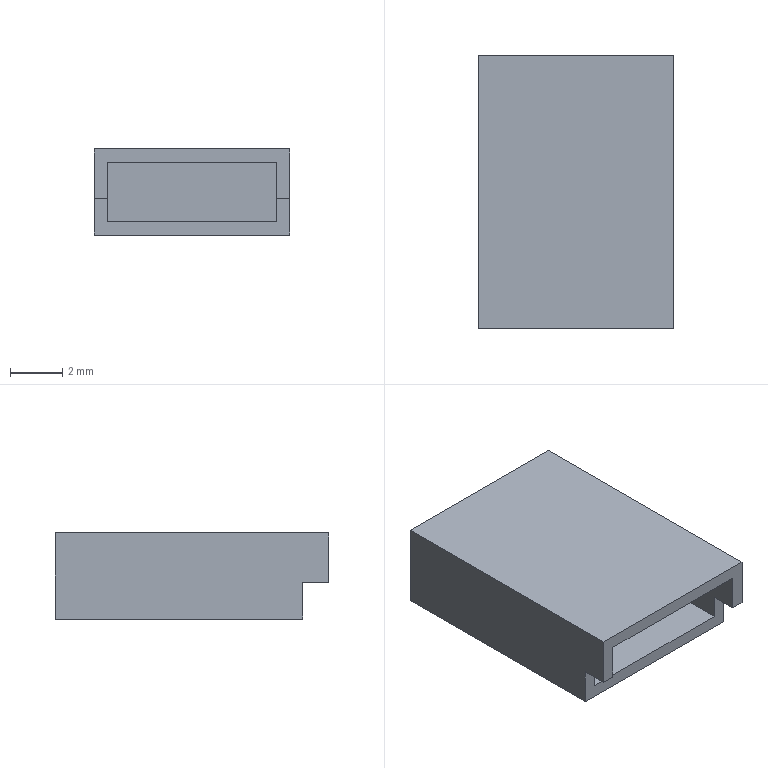Part | SolidWorks | features BaseBody 1 | 1 solid | 14 faces | box 7.5 x 10.5 x 3.3 mm | volume 105.725 mm3 | plane 14
STEP:
#1=CARTESIAN_POINT('',(-3.75,10.5,0.));
#2=VERTEX_POINT('',#1);
#3=CARTESIAN_POINT('',(-3.75,0.,0.));
#4=VERTEX_POINT('',#3);
#5=CARTESIAN_POINT('',(-3.75,0.,0.));
#6=DIRECTION('',(0.,-1.,0.));
#7=VECTOR('',#6,1000.);
#8=LINE('',#5,#7);
#9=EDGE_CURVE('',#2,#4,#8,.T.);
#10=ORIENTED_EDGE('',*,*,#9,.T.);
#11=CARTESIAN_POINT('',(3.75,0.,0.));
#12=VERTEX_POINT('',#11);
#13=CARTESIAN_POINT('',(-3.75,0.,0.));
#14=DIRECTION('',(1.,0.,0.));
#15=VECTOR('',#14,1000.);
#16=LINE('',#13,#15);
#17=EDGE_CURVE('',#4,#12,#16,.T.);
#18=ORIENTED_EDGE('',*,*,#17,.T.);
#19=CARTESIAN_POINT('',(3.75,10.5,0.));
#20=VERTEX_POINT('',#19);
#21=CARTESIAN_POINT('',(3.75,0.,0.));
#22=DIRECTION('',(0.,1.,0.));
#23=VECTOR('',#22,1000.);
#24=LINE('',#21,#23);
#25=EDGE_CURVE('',#12,#20,#24,.T.);
#26=ORIENTED_EDGE('',*,*,#25,.T.);
#27=CARTESIAN_POINT('',(-3.75,10.5,0.));
#28=DIRECTION('',(-1.,0.,0.));
#29=VECTOR('',#28,1000.);
#30=LINE('',#27,#29);
#31=EDGE_CURVE('',#20,#2,#30,.T.);
#32=ORIENTED_EDGE('',*,*,#31,.T.);
#33=EDGE_LOOP('',(#10,#18,#26,#32));
#34=FACE_OUTER_BOUND('',#33,.T.);
#35=CARTESIAN_POINT('',(-3.75,0.,0.));
#36=DIRECTION('',(0.,0.,1.));
#37=DIRECTION('',(1.,0.,0.));
#38=AXIS2_PLACEMENT_3D('',#35,#36,#37);
#39=PLANE('',#38);
#40=ADVANCED_FACE('',(#34),#39,.T.);
#41=CARTESIAN_POINT('',(3.25,0.,-0.5));
#42=VERTEX_POINT('',#41);
#43=CARTESIAN_POINT('',(-3.25,0.,-0.5));
#44=VERTEX_POINT('',#43);
#45=CARTESIAN_POINT('',(0.,0.,-0.5));
#46=DIRECTION('',(-1.,0.,0.));
#47=VECTOR('',#46,1000.);
#48=LINE('',#45,#47);
#49=EDGE_CURVE('',#42,#44,#48,.T.);
#50=ORIENTED_EDGE('',*,*,#49,.F.);
#51=CARTESIAN_POINT('',(3.25,0.,-1.9));
#52=VERTEX_POINT('',#51);
#53=CARTESIAN_POINT('',(3.25,0.,0.));
#54=DIRECTION('',(0.,0.,-1.));
#55=VECTOR('',#54,1000.);
#56=LINE('',#53,#55);
#57=EDGE_CURVE('',#42,#52,#56,.T.);
#58=ORIENTED_EDGE('',*,*,#57,.T.);
#59=CARTESIAN_POINT('',(3.75,0.,-1.9));
#60=VERTEX_POINT('',#59);
#61=CARTESIAN_POINT('',(0.,0.,-1.9));
#62=DIRECTION('',(-1.,0.,0.));
#63=VECTOR('',#62,1000.);
#64=LINE('',#61,#63);
#65=EDGE_CURVE('',#60,#52,#64,.T.);
#66=ORIENTED_EDGE('',*,*,#65,.F.);
#67=CARTESIAN_POINT('',(3.75,0.,0.));
#68=DIRECTION('',(0.,0.,-1.));
#69=VECTOR('',#68,1000.);
#70=LINE('',#67,#69);
#71=EDGE_CURVE('',#12,#60,#70,.T.);
#72=ORIENTED_EDGE('',*,*,#71,.F.);
#73=ORIENTED_EDGE('',*,*,#17,.F.);
#74=CARTESIAN_POINT('',(-3.75,0.,-1.9));
#75=VERTEX_POINT('',#74);
#76=CARTESIAN_POINT('',(-3.75,0.,0.));
#77=DIRECTION('',(0.,0.,1.));
#78=VECTOR('',#77,1000.);
#79=LINE('',#76,#78);
#80=EDGE_CURVE('',#75,#4,#79,.T.);
#81=ORIENTED_EDGE('',*,*,#80,.F.);
#82=CARTESIAN_POINT('',(-3.25,0.,-1.9));
#83=VERTEX_POINT('',#82);
#84=CARTESIAN_POINT('',(0.,0.,-1.9));
#85=DIRECTION('',(-1.,0.,0.));
#86=VECTOR('',#85,1000.);
#87=LINE('',#84,#86);
#88=EDGE_CURVE('',#83,#75,#87,.T.);
#89=ORIENTED_EDGE('',*,*,#88,.F.);
#90=CARTESIAN_POINT('',(-3.25,0.,-3.3));
#91=DIRECTION('',(0.,0.,1.));
#92=VECTOR('',#91,1000.);
#93=LINE('',#90,#92);
#94=EDGE_CURVE('',#83,#44,#93,.T.);
#95=ORIENTED_EDGE('',*,*,#94,.T.);
#96=EDGE_LOOP('',(#50,#58,#66,#72,#73,#81,#89,#95));
#97=FACE_OUTER_BOUND('',#96,.T.);
#98=CARTESIAN_POINT('',(0.,0.,0.));
#99=DIRECTION('',(0.,1.,0.));
#100=DIRECTION('',(0.,0.,1.));
#101=AXIS2_PLACEMENT_3D('',#98,#99,#100);
#102=PLANE('',#101);
#103=ADVANCED_FACE('',(#97),#102,.F.);
#104=CARTESIAN_POINT('',(-3.75,10.5,-3.3));
#105=VERTEX_POINT('',#104);
#106=CARTESIAN_POINT('',(-3.75,1.,-3.3));
#107=VERTEX_POINT('',#106);
#108=CARTESIAN_POINT('',(-3.75,0.,-3.3));
#109=DIRECTION('',(0.,-1.,0.));
#110=VECTOR('',#109,1000.);
#111=LINE('',#108,#110);
#112=EDGE_CURVE('',#105,#107,#111,.T.);
#113=ORIENTED_EDGE('',*,*,#112,.T.);
#114=CARTESIAN_POINT('',(-3.75,1.,-1.9));
#115=VERTEX_POINT('',#114);
#116=CARTESIAN_POINT('',(-3.75,1.,-3.3));
#117=DIRECTION('',(0.,0.,1.));
#118=VECTOR('',#117,1000.);
#119=LINE('',#116,#118);
#120=EDGE_CURVE('',#107,#115,#119,.T.);
#121=ORIENTED_EDGE('',*,*,#120,.T.);
#122=CARTESIAN_POINT('',(-3.75,0.,-1.9));
#123=DIRECTION('',(0.,-1.,0.));
#124=VECTOR('',#123,1000.);
#125=LINE('',#122,#124);
#126=EDGE_CURVE('',#115,#75,#125,.T.);
#127=ORIENTED_EDGE('',*,*,#126,.T.);
#128=ORIENTED_EDGE('',*,*,#80,.T.);
#129=ORIENTED_EDGE('',*,*,#9,.F.);
#130=CARTESIAN_POINT('',(-3.75,10.5,-3.3));
#131=DIRECTION('',(0.,0.,-1.));
#132=VECTOR('',#131,1000.);
#133=LINE('',#130,#132);
#134=EDGE_CURVE('',#2,#105,#133,.T.);
#135=ORIENTED_EDGE('',*,*,#134,.T.);
#136=EDGE_LOOP('',(#113,#121,#127,#128,#129,#135));
#137=FACE_OUTER_BOUND('',#136,.T.);
#138=CARTESIAN_POINT('',(-3.75,0.,-3.3));
#139=DIRECTION('',(-1.,0.,0.));
#140=DIRECTION('',(0.,0.,1.));
#141=AXIS2_PLACEMENT_3D('',#138,#139,#140);
#142=PLANE('',#141);
#143=ADVANCED_FACE('',(#137),#142,.T.);
#144=CARTESIAN_POINT('',(3.75,10.5,-3.3));
#145=VERTEX_POINT('',#144);
#146=CARTESIAN_POINT('',(0.,10.5,-3.3));
#147=DIRECTION('',(-1.,0.,0.));
#148=VECTOR('',#147,1000.);
#149=LINE('',#146,#148);
#150=EDGE_CURVE('',#145,#105,#149,.T.);
#151=ORIENTED_EDGE('',*,*,#150,.T.);
#152=ORIENTED_EDGE('',*,*,#134,.F.);
#153=ORIENTED_EDGE('',*,*,#31,.F.);
#154=CARTESIAN_POINT('',(3.75,10.5,0.));
#155=DIRECTION('',(0.,0.,-1.));
#156=VECTOR('',#155,1000.);
#157=LINE('',#154,#156);
#158=EDGE_CURVE('',#20,#145,#157,.T.);
#159=ORIENTED_EDGE('',*,*,#158,.T.);
#160=EDGE_LOOP('',(#151,#152,#153,#159));
#161=FACE_OUTER_BOUND('',#160,.T.);
#162=CARTESIAN_POINT('',(0.,10.5,0.));
#163=DIRECTION('',(0.,1.,0.));
#164=DIRECTION('',(0.,0.,1.));
#165=AXIS2_PLACEMENT_3D('',#162,#163,#164);
#166=PLANE('',#165);
#167=ADVANCED_FACE('',(#161),#166,.T.);
#168=CARTESIAN_POINT('',(3.75,1.,-1.9));
#169=VERTEX_POINT('',#168);
#170=CARTESIAN_POINT('',(3.75,0.,-1.9));
#171=DIRECTION('',(0.,1.,0.));
#172=VECTOR('',#171,1000.);
#173=LINE('',#170,#172);
#174=EDGE_CURVE('',#60,#169,#173,.T.);
#175=ORIENTED_EDGE('',*,*,#174,.T.);
#176=CARTESIAN_POINT('',(3.75,1.,-3.3));
#177=VERTEX_POINT('',#176);
#178=CARTESIAN_POINT('',(3.75,1.,-3.3));
#179=DIRECTION('',(0.,0.,-1.));
#180=VECTOR('',#179,1000.);
#181=LINE('',#178,#180);
#182=EDGE_CURVE('',#169,#177,#181,.T.);
#183=ORIENTED_EDGE('',*,*,#182,.T.);
#184=CARTESIAN_POINT('',(3.75,0.,-3.3));
#185=DIRECTION('',(0.,1.,0.));
#186=VECTOR('',#185,1000.);
#187=LINE('',#184,#186);
#188=EDGE_CURVE('',#177,#145,#187,.T.);
#189=ORIENTED_EDGE('',*,*,#188,.T.);
#190=ORIENTED_EDGE('',*,*,#158,.F.);
#191=ORIENTED_EDGE('',*,*,#25,.F.);
#192=ORIENTED_EDGE('',*,*,#71,.T.);
#193=EDGE_LOOP('',(#175,#183,#189,#190,#191,#192));
#194=FACE_OUTER_BOUND('',#193,.T.);
#195=CARTESIAN_POINT('',(3.75,0.,0.));
#196=DIRECTION('',(1.,0.,0.));
#197=DIRECTION('',(0.,0.,-1.));
#198=AXIS2_PLACEMENT_3D('',#195,#196,#197);
#199=PLANE('',#198);
#200=ADVANCED_FACE('',(#194),#199,.T.);
#201=CARTESIAN_POINT('',(3.25,10.,-0.5));
#202=VERTEX_POINT('',#201);
#203=CARTESIAN_POINT('',(-3.25,10.,-0.5));
#204=VERTEX_POINT('',#203);
#205=CARTESIAN_POINT('',(-3.75,10.,-0.5));
#206=DIRECTION('',(-1.,0.,0.));
#207=VECTOR('',#206,1000.);
#208=LINE('',#205,#207);
#209=EDGE_CURVE('',#202,#204,#208,.T.);
#210=ORIENTED_EDGE('',*,*,#209,.F.);
#211=CARTESIAN_POINT('',(3.25,0.,-0.5));
#212=DIRECTION('',(0.,1.,0.));
#213=VECTOR('',#212,1000.);
#214=LINE('',#211,#213);
#215=EDGE_CURVE('',#42,#202,#214,.T.);
#216=ORIENTED_EDGE('',*,*,#215,.F.);
#217=ORIENTED_EDGE('',*,*,#49,.T.);
#218=CARTESIAN_POINT('',(-3.25,0.,-0.5));
#219=DIRECTION('',(0.,-1.,0.));
#220=VECTOR('',#219,1000.);
#221=LINE('',#218,#220);
#222=EDGE_CURVE('',#204,#44,#221,.T.);
#223=ORIENTED_EDGE('',*,*,#222,.F.);
#224=EDGE_LOOP('',(#210,#216,#217,#223));
#225=FACE_OUTER_BOUND('',#224,.T.);
#226=CARTESIAN_POINT('',(-3.75,0.,-0.5));
#227=DIRECTION('',(0.,0.,1.));
#228=DIRECTION('',(1.,0.,0.));
#229=AXIS2_PLACEMENT_3D('',#226,#227,#228);
#230=PLANE('',#229);
#231=ADVANCED_FACE('',(#225),#230,.F.);
#232=CARTESIAN_POINT('',(3.25,1.,-1.9));
#233=VERTEX_POINT('',#232);
#234=CARTESIAN_POINT('',(3.25,1.,-1.9));
#235=DIRECTION('',(0.,-1.,0.));
#236=VECTOR('',#235,1000.);
#237=LINE('',#234,#236);
#238=EDGE_CURVE('',#233,#52,#237,.T.);
#239=ORIENTED_EDGE('',*,*,#238,.F.);
#240=CARTESIAN_POINT('',(3.75,1.,-1.9));
#241=DIRECTION('',(1.,0.,0.));
#242=VECTOR('',#241,1000.);
#243=LINE('',#240,#242);
#244=EDGE_CURVE('',#233,#169,#243,.T.);
#245=ORIENTED_EDGE('',*,*,#244,.T.);
#246=ORIENTED_EDGE('',*,*,#174,.F.);
#247=ORIENTED_EDGE('',*,*,#65,.T.);
#248=EDGE_LOOP('',(#239,#245,#246,#247));
#249=FACE_OUTER_BOUND('',#248,.T.);
#250=CARTESIAN_POINT('',(3.75,1.,-1.9));
#251=DIRECTION('',(0.,0.,1.));
#252=DIRECTION('',(1.,0.,0.));
#253=AXIS2_PLACEMENT_3D('',#250,#251,#252);
#254=PLANE('',#253);
#255=ADVANCED_FACE('',(#249),#254,.F.);
#256=CARTESIAN_POINT('',(-3.25,1.,-1.9));
#257=VERTEX_POINT('',#256);
#258=CARTESIAN_POINT('',(3.75,1.,-1.9));
#259=DIRECTION('',(1.,0.,0.));
#260=VECTOR('',#259,1000.);
#261=LINE('',#258,#260);
#262=EDGE_CURVE('',#115,#257,#261,.T.);
#263=ORIENTED_EDGE('',*,*,#262,.T.);
#264=CARTESIAN_POINT('',(-3.25,1.,-1.9));
#265=DIRECTION('',(0.,1.,0.));
#266=VECTOR('',#265,1000.);
#267=LINE('',#264,#266);
#268=EDGE_CURVE('',#83,#257,#267,.T.);
#269=ORIENTED_EDGE('',*,*,#268,.F.);
#270=ORIENTED_EDGE('',*,*,#88,.T.);
#271=ORIENTED_EDGE('',*,*,#126,.F.);
#272=EDGE_LOOP('',(#263,#269,#270,#271));
#273=FACE_OUTER_BOUND('',#272,.T.);
#274=CARTESIAN_POINT('',(3.75,1.,-1.9));
#275=DIRECTION('',(0.,0.,1.));
#276=DIRECTION('',(1.,0.,0.));
#277=AXIS2_PLACEMENT_3D('',#274,#275,#276);
#278=PLANE('',#277);
#279=ADVANCED_FACE('',(#273),#278,.F.);
#280=ORIENTED_EDGE('',*,*,#188,.F.);
#281=CARTESIAN_POINT('',(3.75,1.,-3.3));
#282=DIRECTION('',(-1.,0.,0.));
#283=VECTOR('',#282,1000.);
#284=LINE('',#281,#283);
#285=EDGE_CURVE('',#177,#107,#284,.T.);
#286=ORIENTED_EDGE('',*,*,#285,.T.);
#287=ORIENTED_EDGE('',*,*,#112,.F.);
#288=ORIENTED_EDGE('',*,*,#150,.F.);
#289=EDGE_LOOP('',(#280,#286,#287,#288));
#290=FACE_OUTER_BOUND('',#289,.T.);
#291=CARTESIAN_POINT('',(3.75,0.,-3.3));
#292=DIRECTION('',(0.,0.,-1.));
#293=DIRECTION('',(-1.,0.,0.));
#294=AXIS2_PLACEMENT_3D('',#291,#292,#293);
#295=PLANE('',#294);
#296=ADVANCED_FACE('',(#290),#295,.T.);
#297=CARTESIAN_POINT('',(-3.25,10.,-2.8));
#298=VERTEX_POINT('',#297);
#299=CARTESIAN_POINT('',(-3.25,10.,-3.3));
#300=DIRECTION('',(0.,0.,-1.));
#301=VECTOR('',#300,1000.);
#302=LINE('',#299,#301);
#303=EDGE_CURVE('',#204,#298,#302,.T.);
#304=ORIENTED_EDGE('',*,*,#303,.F.);
#305=ORIENTED_EDGE('',*,*,#222,.T.);
#306=ORIENTED_EDGE('',*,*,#94,.F.);
#307=ORIENTED_EDGE('',*,*,#268,.T.);
#308=CARTESIAN_POINT('',(-3.25,1.,-2.8));
#309=VERTEX_POINT('',#308);
#310=CARTESIAN_POINT('',(-3.25,1.,-3.3));
#311=DIRECTION('',(0.,0.,1.));
#312=VECTOR('',#311,1000.);
#313=LINE('',#310,#312);
#314=EDGE_CURVE('',#309,#257,#313,.T.);
#315=ORIENTED_EDGE('',*,*,#314,.F.);
#316=CARTESIAN_POINT('',(-3.25,0.,-2.8));
#317=DIRECTION('',(0.,-1.,0.));
#318=VECTOR('',#317,1000.);
#319=LINE('',#316,#318);
#320=EDGE_CURVE('',#298,#309,#319,.T.);
#321=ORIENTED_EDGE('',*,*,#320,.F.);
#322=EDGE_LOOP('',(#304,#305,#306,#307,#315,#321));
#323=FACE_OUTER_BOUND('',#322,.T.);
#324=CARTESIAN_POINT('',(-3.25,0.,-3.3));
#325=DIRECTION('',(-1.,0.,0.));
#326=DIRECTION('',(0.,0.,1.));
#327=AXIS2_PLACEMENT_3D('',#324,#325,#326);
#328=PLANE('',#327);
#329=ADVANCED_FACE('',(#323),#328,.F.);
#330=CARTESIAN_POINT('',(3.25,10.,-2.8));
#331=VERTEX_POINT('',#330);
#332=CARTESIAN_POINT('',(3.25,10.,0.));
#333=DIRECTION('',(0.,0.,-1.));
#334=VECTOR('',#333,1000.);
#335=LINE('',#332,#334);
#336=EDGE_CURVE('',#202,#331,#335,.T.);
#337=ORIENTED_EDGE('',*,*,#336,.F.);
#338=ORIENTED_EDGE('',*,*,#209,.T.);
#339=ORIENTED_EDGE('',*,*,#303,.T.);
#340=CARTESIAN_POINT('',(0.,10.,-2.8));
#341=DIRECTION('',(-1.,0.,0.));
#342=VECTOR('',#341,1000.);
#343=LINE('',#340,#342);
#344=EDGE_CURVE('',#331,#298,#343,.T.);
#345=ORIENTED_EDGE('',*,*,#344,.F.);
#346=EDGE_LOOP('',(#337,#338,#339,#345));
#347=FACE_OUTER_BOUND('',#346,.T.);
#348=CARTESIAN_POINT('',(0.,10.,0.));
#349=DIRECTION('',(0.,1.,0.));
#350=DIRECTION('',(0.,0.,1.));
#351=AXIS2_PLACEMENT_3D('',#348,#349,#350);
#352=PLANE('',#351);
#353=ADVANCED_FACE('',(#347),#352,.F.);
#354=ORIENTED_EDGE('',*,*,#57,.F.);
#355=ORIENTED_EDGE('',*,*,#215,.T.);
#356=ORIENTED_EDGE('',*,*,#336,.T.);
#357=CARTESIAN_POINT('',(3.25,1.,-2.8));
#358=VERTEX_POINT('',#357);
#359=CARTESIAN_POINT('',(3.25,0.,-2.8));
#360=DIRECTION('',(0.,1.,0.));
#361=VECTOR('',#360,1000.);
#362=LINE('',#359,#361);
#363=EDGE_CURVE('',#358,#331,#362,.T.);
#364=ORIENTED_EDGE('',*,*,#363,.F.);
#365=CARTESIAN_POINT('',(3.25,1.,0.));
#366=DIRECTION('',(0.,0.,-1.));
#367=VECTOR('',#366,1000.);
#368=LINE('',#365,#367);
#369=EDGE_CURVE('',#233,#358,#368,.T.);
#370=ORIENTED_EDGE('',*,*,#369,.F.);
#371=ORIENTED_EDGE('',*,*,#238,.T.);
#372=EDGE_LOOP('',(#354,#355,#356,#364,#370,#371));
#373=FACE_OUTER_BOUND('',#372,.T.);
#374=CARTESIAN_POINT('',(3.25,0.,0.));
#375=DIRECTION('',(1.,0.,0.));
#376=DIRECTION('',(0.,0.,-1.));
#377=AXIS2_PLACEMENT_3D('',#374,#375,#376);
#378=PLANE('',#377);
#379=ADVANCED_FACE('',(#373),#378,.F.);
#380=ORIENTED_EDGE('',*,*,#182,.F.);
#381=ORIENTED_EDGE('',*,*,#244,.F.);
#382=ORIENTED_EDGE('',*,*,#369,.T.);
#383=CARTESIAN_POINT('',(3.75,1.,-2.8));
#384=DIRECTION('',(1.,0.,0.));
#385=VECTOR('',#384,1000.);
#386=LINE('',#383,#385);
#387=EDGE_CURVE('',#309,#358,#386,.T.);
#388=ORIENTED_EDGE('',*,*,#387,.F.);
#389=ORIENTED_EDGE('',*,*,#314,.T.);
#390=ORIENTED_EDGE('',*,*,#262,.F.);
#391=ORIENTED_EDGE('',*,*,#120,.F.);
#392=ORIENTED_EDGE('',*,*,#285,.F.);
#393=EDGE_LOOP('',(#380,#381,#382,#388,#389,#390,#391,#392));
#394=FACE_OUTER_BOUND('',#393,.T.);
#395=CARTESIAN_POINT('',(3.75,1.,-3.3));
#396=DIRECTION('',(0.,1.,0.));
#397=DIRECTION('',(0.,0.,1.));
#398=AXIS2_PLACEMENT_3D('',#395,#396,#397);
#399=PLANE('',#398);
#400=ADVANCED_FACE('',(#394),#399,.F.);
#401=ORIENTED_EDGE('',*,*,#344,.T.);
#402=ORIENTED_EDGE('',*,*,#320,.T.);
#403=ORIENTED_EDGE('',*,*,#387,.T.);
#404=ORIENTED_EDGE('',*,*,#363,.T.);
#405=EDGE_LOOP('',(#401,#402,#403,#404));
#406=FACE_OUTER_BOUND('',#405,.T.);
#407=CARTESIAN_POINT('',(3.75,0.,-2.8));
#408=DIRECTION('',(0.,0.,-1.));
#409=DIRECTION('',(-1.,0.,0.));
#410=AXIS2_PLACEMENT_3D('',#407,#408,#409);
#411=PLANE('',#410);
#412=ADVANCED_FACE('',(#406),#411,.F.);
#413=CLOSED_SHELL('',(#40,#103,#143,#167,#200,#231,#255,#279,#296,#329,#353,#379,#400,#412));
#414=MANIFOLD_SOLID_BREP('',#413);
#415=CARTESIAN_POINT('',(0.,0.,0.));
#416=DIRECTION('',(0.,0.,1.));
#417=DIRECTION('',(1.,0.,0.));
#418=AXIS2_PLACEMENT_3D('',#415,#416,#417);
#419=(LENGTH_UNIT()NAMED_UNIT(*)SI_UNIT(.MILLI.,.METRE.));
#420=UNCERTAINTY_MEASURE_WITH_UNIT(LENGTH_MEASURE(0.00001),#419,'','');
#421=(NAMED_UNIT(*)PLANE_ANGLE_UNIT()SI_UNIT($,.RADIAN.));
#422=(NAMED_UNIT(*)SI_UNIT($,.STERADIAN.)SOLID_ANGLE_UNIT());
#423=(GEOMETRIC_REPRESENTATION_CONTEXT(3)GLOBAL_UNCERTAINTY_ASSIGNED_CONTEXT((#420))GLOBAL_UNIT_ASSIGNED_CONTEXT((#419,#421,#422))REPRESENTATION_CONTEXT('',''));
#424=ADVANCED_BREP_SHAPE_REPRESENTATION('',(#414,#418),#423);